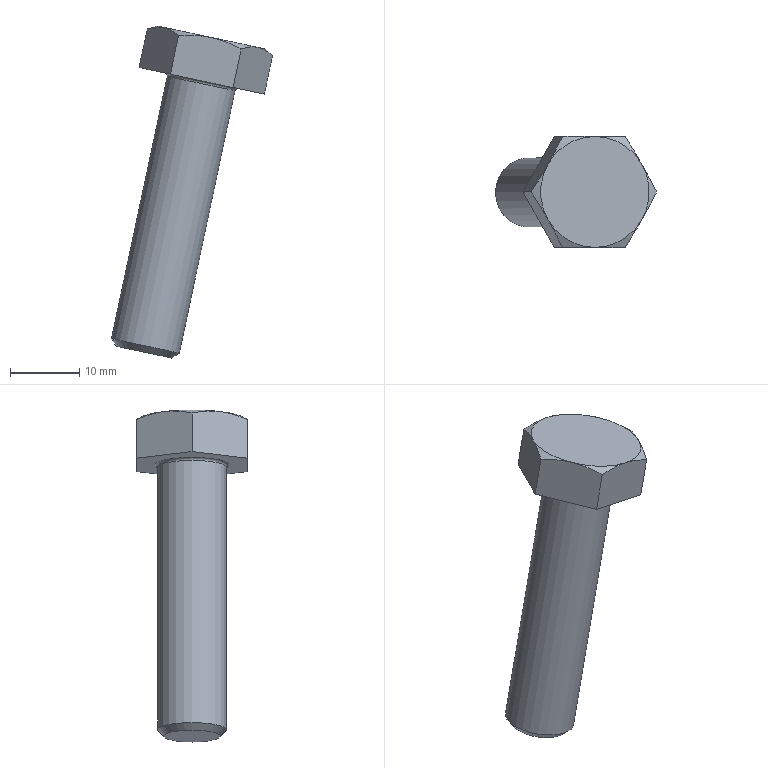Part | STEP file | 8901-M1040B (bolt M10×40) | 1 solid | 18 faces | box 23.234 x 16 x 47.898 mm | volume 4545 mm3 | plane 9 | cone 7 | cylinder 1 | torus 1 | commonest cylinder face diameters 10 x1